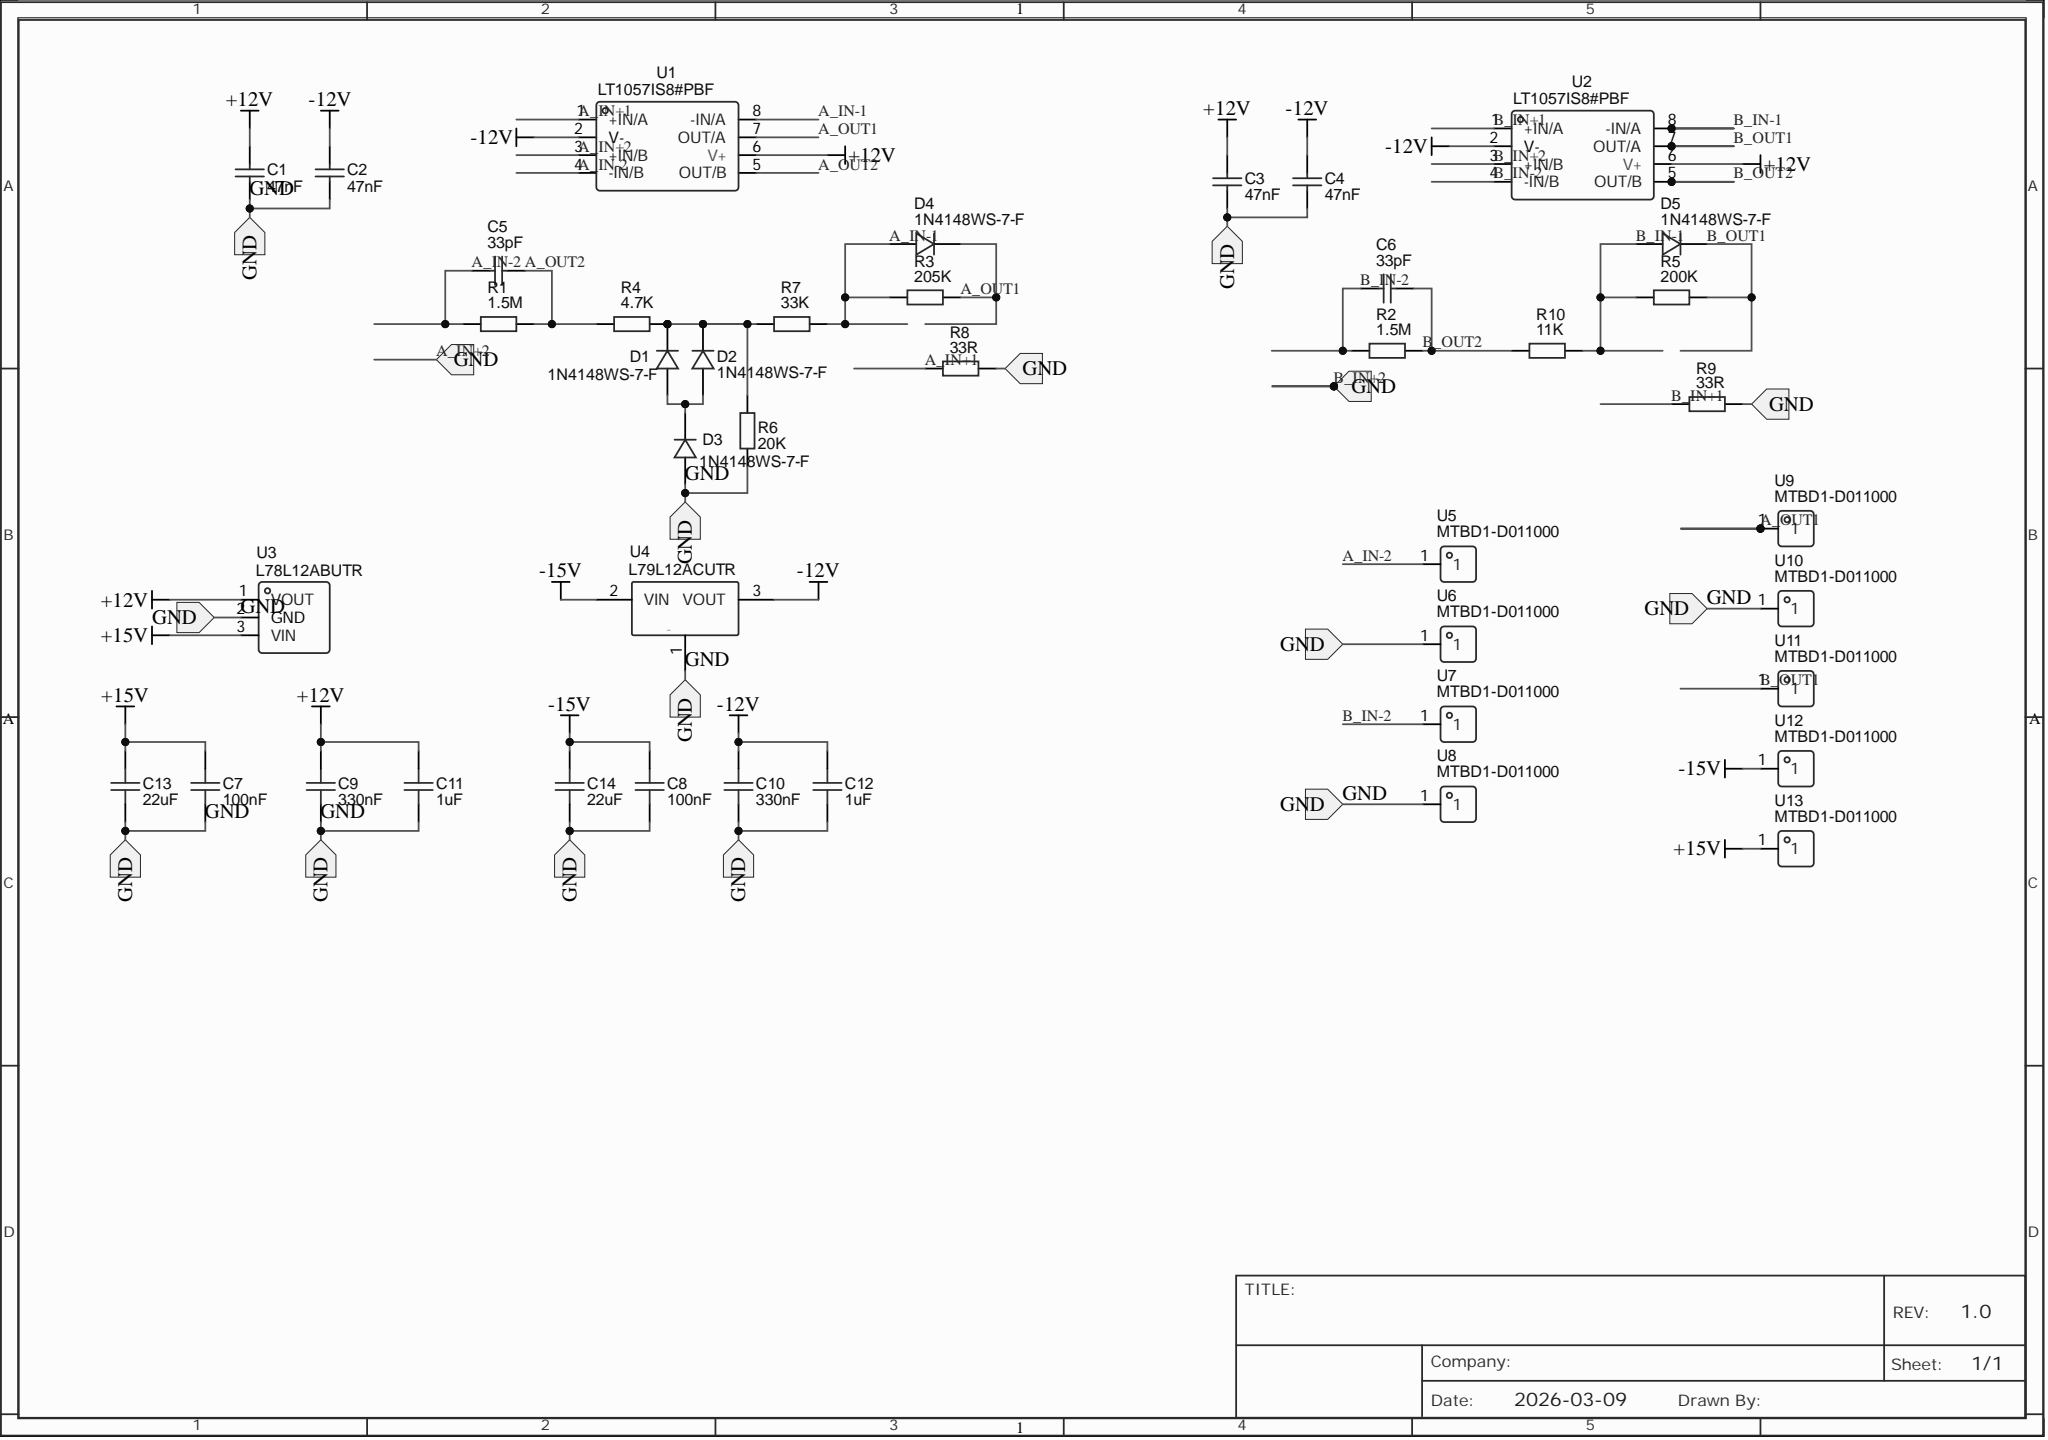Circuit board | Altium Designer | 42 parts | 17 nets
Bill of materials:
Comment,Description,Designator,Footprint,LibRef,Quantity
"47nF","","C1, C2, C3, C4","C0603","CL10B473KB8NNNC","4"
"33pF","","C5, C6","C0603","CL10C330JB8NNNC","2"
"100nF","","C7, C8","C0603","CGA0603X7R104K500JT","2"
"330nF","","C9, C10","C0603","FCC0603B334K500CT","2"
"1uF","","C11, C12","C0603","CGA0805X7R105K500MT","2"
"22uF","","C13, C14","C1210","CL32B226KAJNNNE","2"
"1N4148WS-7-F","","D1, D2, D3, D4, D5","SOD-323_L1.8-W1.3-LS2.5-RD","1N4148WS-7-F","5"
"1.5M","","R1, R2","R0603","0603WAF1504T5E","2"
"205K","","R3","R0603","0603WAF1504T5E","1"
"4.7K","","R4","R0603","0603WAF1504T5E","1"
"200K","","R5","R0603","0603WAF1504T5E","1"
"20K","","R6","R0603","0603WAF1504T5E","1"
"33K","","R7","R0603","0603WAF1504T5E","1"
"33R","","R8, R9","R0603","0603WAF1504T5E","2"
"11K","","R10","R0603","0603WAF1504T5E","1"
"LT1057IS8#PBF","","U1, U2","SOIC-8_L5.0-W4.0-P1.27-LS6.0-BL","LT1057IS8#PBF","2"
"L78L12ABUTR","","U3","SOT-89-3_L4.5-W2.5-P1.50-LS4.2-BR","L78L12ABUTR","1"
"L79L12ACUTR","","U4","SOT-89-3_L4.5-W2.5-P1.50-LS4.2-TL","L79L12ACUTR","1"
"MTBD1-D011000","","U5, U6, U7, U8, U9, U10, U11, U12, U13","CR100","MTBD1-D011000","9"
Netlist (Protel format):
[
C1
C0603
47nF



]
[
C2
C0603
47nF



]
[
C3
C0603
47nF



]
[
C4
C0603
47nF



]
[
C5
C0603
33pF



]
[
C6
C0603
33pF



]
[
C7
C0603
100nF



]
[
C8
C0603
100nF



]
[
C9
C0603
330nF



]
[
C10
C0603
330nF



]
[
C11
C0603
1uF



]
[
C12
C0603
1uF



]
[
C13
C1210
22uF



]
[
C14
C1210
22uF



]
[
D1
SOD-323_L1.8-W1.3-LS2.5-RD
1N4148WS-7-F



]
[
D2
SOD-323_L1.8-W1.3-LS2.5-RD
1N4148WS-7-F



]
[
D3
SOD-323_L1.8-W1.3-LS2.5-RD
1N4148WS-7-F



]
[
D4
SOD-323_L1.8-W1.3-LS2.5-RD
1N4148WS-7-F



]
[
D5
SOD-323_L1.8-W1.3-LS2.5-RD
1N4148WS-7-F



]
[
R1
R0603
1.5M



]
[
R2
R0603
1.5M



]
[
R3
R0603
205K



]
[
R4
R0603
4.7K



]
[
R5
R0603
200K



]
[
R6
R0603
20K



]
[
R7
R0603
33K



]
[
R8
R0603
33R



]
[
R9
R0603
33R



]
[
R10
R0603
11K



]
[
U1
SOIC-8_L5.0-W4.0-P1.27-LS6.0-BL
LT1057IS8#PBF



]
[
U2
SOIC-8_L5.0-W4.0-P1.27-LS6.0-BL
LT1057IS8#PBF



]
[
U3
SOT-89-3_L4.5-W2.5-P1.50-LS4.2-BR
L78L12ABUTR



]
[
U4
SOT-89-3_L4.5-W2.5-P1.50-LS4.2-TL
L79L12ACUTR



]
[
U5
CR100
MTBD1-D011000



]
[
U6
CR100
MTBD1-D011000



]
[
U7
CR100
MTBD1-D011000



]
[
U8
CR100
MTBD1-D011000



]
[
U9
CR100
MTBD1-D011000



]
[
U10
CR100
MTBD1-D011000



]
[
U11
CR100
MTBD1-D011000



]
[
U12
CR100
MTBD1-D011000



]
[
U13
CR100
MTBD1-D011000



]
(
NetD1_2
D1-2
D2-2
D3-1
)
(
NetD1_1
D1-1
D2-1
R4-2
R6-2
R7-1
)
(
B_OUT2
C6-2
R2-2
R10-1
U2-5
)
(
B_OUT1
D5-1
R5-2
U2-7
U11-1
)
(
B_IN-2
C6-1
R2-1
U2-4
U7-1
)
(
B_IN-1
D5-2
R5-1
R10-2
U2-8
)
(
B_IN+1
R9-1
U2-1
)
(
A_OUT2
C5-2
R1-2
R4-1
U1-5
)
(
A_OUT1
D4-1
R3-2
U1-7
U9-1
)
(
A_IN-2
C5-1
R1-1
U1-4
U5-1
)
(
A_IN-1
D4-2
R3-1
R7-2
U1-8
)
(
A_IN+2
C1-1
C2-1
C3-1
C4-1
C7-1
C8-1
C9-1
C10-1
C11-1
C12-1
C13-2
C14-2
D3-2
R6-1
R8-2
R9-2
U1-3
U2-3
U3-2
U4-1
U6-1
U8-1
U10-1
)
(
A_IN+1
R8-1
U1-1
)
(
-15V
C8-2
C14-1
U4-2
U12-1
)
(
-12V
C2-2
C4-2
C10-2
C12-2
U1-2
U2-2
U4-3
)
(
+15V
C7-2
C13-1
U3-3
U13-1
)
(
+12V
C1-2
C3-2
C9-2
C11-2
U1-6
U2-6
U3-1
)